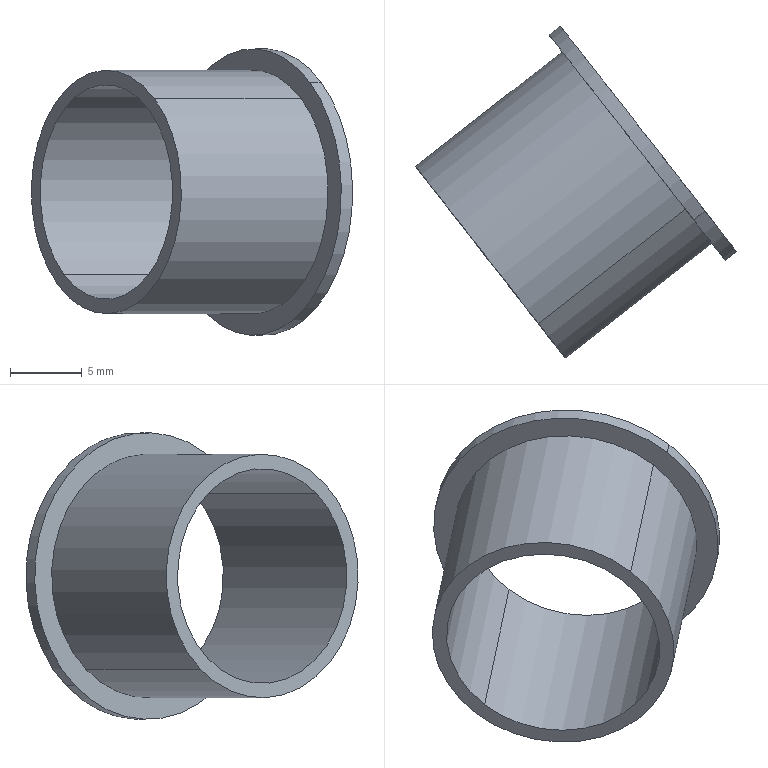Part | SolidWorks | features BaseBody 1 | 1 solid | 9 faces | box 22.422 x 23.197 x 20 mm | volume 790.896 mm3 | cylinder 6 | plane 3 | commonest cylinder face diameters 15 x2 17 x2 20 x2
STEP:
#1=CARTESIAN_POINT('',(6.767,90.458,77.91));
#2=VERTEX_POINT('',#1);
#3=CARTESIAN_POINT('',(-1.148,100.588,62.59));
#4=VERTEX_POINT('',#3);
#5=CARTESIAN_POINT('',(2.809,95.523,70.25));
#6=DIRECTION('',(-0.788,-0.6157,0.));
#7=DIRECTION('',(0.3957,-0.5065,0.766));
#8=AXIS2_PLACEMENT_3D('',#5,#6,#7);
#9=CIRCLE('',#8,10.);
#10=EDGE_CURVE('',#2,#4,#9,.T.);
#11=ORIENTED_EDGE('',*,*,#10,.F.);
#12=CARTESIAN_POINT('',(7.555,91.074,77.91));
#13=VERTEX_POINT('',#12);
#14=CARTESIAN_POINT('',(6.767,90.458,77.91));
#15=DIRECTION('',(0.788,0.6157,0.));
#16=VECTOR('',#15,1000.);
#17=LINE('',#14,#16);
#18=EDGE_CURVE('',#2,#13,#17,.T.);
#19=ORIENTED_EDGE('',*,*,#18,.T.);
#20=CARTESIAN_POINT('',(-0.36,101.204,62.59));
#21=VERTEX_POINT('',#20);
#22=CARTESIAN_POINT('',(3.597,96.139,70.25));
#23=DIRECTION('',(-0.788,-0.6157,0.));
#24=DIRECTION('',(0.3957,-0.5065,0.766));
#25=AXIS2_PLACEMENT_3D('',#22,#23,#24);
#26=CIRCLE('',#25,10.);
#27=EDGE_CURVE('',#13,#21,#26,.T.);
#28=ORIENTED_EDGE('',*,*,#27,.T.);
#29=CARTESIAN_POINT('',(-1.148,100.588,62.59));
#30=DIRECTION('',(0.788,0.6157,0.));
#31=VECTOR('',#30,1000.);
#32=LINE('',#29,#31);
#33=EDGE_CURVE('',#4,#21,#32,.T.);
#34=ORIENTED_EDGE('',*,*,#33,.F.);
#35=EDGE_LOOP('',(#11,#19,#28,#34));
#36=FACE_OUTER_BOUND('',#35,.T.);
#37=CARTESIAN_POINT('',(2.809,95.523,70.25));
#38=DIRECTION('',(0.788,0.6157,0.));
#39=DIRECTION('',(-0.3957,0.5065,-0.766));
#40=AXIS2_PLACEMENT_3D('',#37,#38,#39);
#41=CYLINDRICAL_SURFACE('',#40,10.);
#42=ADVANCED_FACE('',(#36),#41,.T.);
#43=CARTESIAN_POINT('',(-4.071,83.214,76.761));
#44=VERTEX_POINT('',#43);
#45=CARTESIAN_POINT('',(-10.799,91.825,63.739));
#46=VERTEX_POINT('',#45);
#47=CARTESIAN_POINT('',(-7.435,87.52,70.25));
#48=DIRECTION('',(-0.788,-0.6157,0.));
#49=DIRECTION('',(0.3957,-0.5065,0.766));
#50=AXIS2_PLACEMENT_3D('',#47,#48,#49);
#51=CIRCLE('',#50,8.5);
#52=EDGE_CURVE('',#44,#46,#51,.T.);
#53=ORIENTED_EDGE('',*,*,#52,.F.);
#54=CARTESIAN_POINT('',(6.173,91.218,76.761));
#55=VERTEX_POINT('',#54);
#56=CARTESIAN_POINT('',(-4.071,83.214,76.761));
#57=DIRECTION('',(0.788,0.6157,0.));
#58=VECTOR('',#57,1000.);
#59=LINE('',#56,#58);
#60=EDGE_CURVE('',#44,#55,#59,.T.);
#61=ORIENTED_EDGE('',*,*,#60,.T.);
#62=CARTESIAN_POINT('',(-0.5544,99.829,63.739));
#63=VERTEX_POINT('',#62);
#64=CARTESIAN_POINT('',(2.809,95.523,70.25));
#65=DIRECTION('',(-0.788,-0.6157,0.));
#66=DIRECTION('',(0.3957,-0.5065,0.766));
#67=AXIS2_PLACEMENT_3D('',#64,#65,#66);
#68=CIRCLE('',#67,8.5);
#69=EDGE_CURVE('',#55,#63,#68,.T.);
#70=ORIENTED_EDGE('',*,*,#69,.T.);
#71=CARTESIAN_POINT('',(-10.799,91.825,63.739));
#72=DIRECTION('',(0.788,0.6157,0.));
#73=VECTOR('',#72,1000.);
#74=LINE('',#71,#73);
#75=EDGE_CURVE('',#46,#63,#74,.T.);
#76=ORIENTED_EDGE('',*,*,#75,.F.);
#77=EDGE_LOOP('',(#53,#61,#70,#76));
#78=FACE_OUTER_BOUND('',#77,.T.);
#79=CARTESIAN_POINT('',(-7.435,87.52,70.25));
#80=DIRECTION('',(0.788,0.6157,0.));
#81=DIRECTION('',(-0.3957,0.5065,-0.766));
#82=AXIS2_PLACEMENT_3D('',#79,#80,#81);
#83=CYLINDRICAL_SURFACE('',#82,8.5);
#84=ADVANCED_FACE('',(#78),#83,.T.);
#85=CARTESIAN_POINT('',(0.6293,99.938,64.505));
#86=VERTEX_POINT('',#85);
#87=CARTESIAN_POINT('',(6.565,92.34,75.995));
#88=VERTEX_POINT('',#87);
#89=CARTESIAN_POINT('',(3.597,96.139,70.25));
#90=DIRECTION('',(-0.788,-0.6157,0.));
#91=DIRECTION('',(0.3957,-0.5065,0.766));
#92=AXIS2_PLACEMENT_3D('',#89,#90,#91);
#93=CIRCLE('',#92,7.5);
#94=EDGE_CURVE('',#86,#88,#93,.T.);
#95=ORIENTED_EDGE('',*,*,#94,.F.);
#96=CARTESIAN_POINT('',(-10.403,91.319,64.505));
#97=VERTEX_POINT('',#96);
#98=CARTESIAN_POINT('',(0.6293,99.938,64.505));
#99=DIRECTION('',(-0.788,-0.6157,0.));
#100=VECTOR('',#99,1000.);
#101=LINE('',#98,#100);
#102=EDGE_CURVE('',#86,#97,#101,.T.);
#103=ORIENTED_EDGE('',*,*,#102,.T.);
#104=CARTESIAN_POINT('',(-4.467,83.721,75.995));
#105=VERTEX_POINT('',#104);
#106=CARTESIAN_POINT('',(-7.435,87.52,70.25));
#107=DIRECTION('',(-0.788,-0.6157,0.));
#108=DIRECTION('',(0.3957,-0.5065,0.766));
#109=AXIS2_PLACEMENT_3D('',#106,#107,#108);
#110=CIRCLE('',#109,7.5);
#111=EDGE_CURVE('',#97,#105,#110,.T.);
#112=ORIENTED_EDGE('',*,*,#111,.T.);
#113=CARTESIAN_POINT('',(6.565,92.34,75.995));
#114=DIRECTION('',(-0.788,-0.6157,0.));
#115=VECTOR('',#114,1000.);
#116=LINE('',#113,#115);
#117=EDGE_CURVE('',#88,#105,#116,.T.);
#118=ORIENTED_EDGE('',*,*,#117,.F.);
#119=EDGE_LOOP('',(#95,#103,#112,#118));
#120=FACE_OUTER_BOUND('',#119,.T.);
#121=CARTESIAN_POINT('',(3.597,96.139,70.25));
#122=DIRECTION('',(-0.788,-0.6157,0.));
#123=DIRECTION('',(0.3957,-0.5065,0.766));
#124=AXIS2_PLACEMENT_3D('',#121,#122,#123);
#125=CYLINDRICAL_SURFACE('',#124,7.5);
#126=ADVANCED_FACE('',(#120),#125,.F.);
#127=ORIENTED_EDGE('',*,*,#102,.F.);
#128=CARTESIAN_POINT('',(3.597,96.139,70.25));
#129=DIRECTION('',(-0.788,-0.6157,0.));
#130=DIRECTION('',(0.3957,-0.5065,0.766));
#131=AXIS2_PLACEMENT_3D('',#128,#129,#130);
#132=CIRCLE('',#131,7.5);
#133=EDGE_CURVE('',#88,#86,#132,.T.);
#134=ORIENTED_EDGE('',*,*,#133,.F.);
#135=ORIENTED_EDGE('',*,*,#117,.T.);
#136=CARTESIAN_POINT('',(-7.435,87.52,70.25));
#137=DIRECTION('',(-0.788,-0.6157,0.));
#138=DIRECTION('',(0.3957,-0.5065,0.766));
#139=AXIS2_PLACEMENT_3D('',#136,#137,#138);
#140=CIRCLE('',#139,7.5);
#141=EDGE_CURVE('',#105,#97,#140,.T.);
#142=ORIENTED_EDGE('',*,*,#141,.T.);
#143=EDGE_LOOP('',(#127,#134,#135,#142));
#144=FACE_OUTER_BOUND('',#143,.T.);
#145=CARTESIAN_POINT('',(3.597,96.139,70.25));
#146=DIRECTION('',(-0.788,-0.6157,0.));
#147=DIRECTION('',(0.3957,-0.5065,0.766));
#148=AXIS2_PLACEMENT_3D('',#145,#146,#147);
#149=CYLINDRICAL_SURFACE('',#148,7.5);
#150=ADVANCED_FACE('',(#144),#149,.F.);
#151=CARTESIAN_POINT('',(-7.435,87.52,70.25));
#152=DIRECTION('',(-0.788,-0.6157,0.));
#153=DIRECTION('',(0.3957,-0.5065,0.766));
#154=AXIS2_PLACEMENT_3D('',#151,#152,#153);
#155=CIRCLE('',#154,8.5);
#156=EDGE_CURVE('',#46,#44,#155,.T.);
#157=ORIENTED_EDGE('',*,*,#156,.T.);
#158=ORIENTED_EDGE('',*,*,#52,.T.);
#159=EDGE_LOOP('',(#157,#158));
#160=FACE_OUTER_BOUND('',#159,.T.);
#161=ORIENTED_EDGE('',*,*,#141,.F.);
#162=ORIENTED_EDGE('',*,*,#111,.F.);
#163=EDGE_LOOP('',(#161,#162));
#164=FACE_BOUND('',#163,.T.);
#165=CARTESIAN_POINT('',(-7.435,87.52,70.25));
#166=DIRECTION('',(-0.788,-0.6157,0.));
#167=DIRECTION('',(-0.6157,0.788,0.));
#168=AXIS2_PLACEMENT_3D('',#165,#166,#167);
#169=PLANE('',#168);
#170=ADVANCED_FACE('',(#160,#164),#169,.T.);
#171=ORIENTED_EDGE('',*,*,#60,.F.);
#172=ORIENTED_EDGE('',*,*,#156,.F.);
#173=ORIENTED_EDGE('',*,*,#75,.T.);
#174=CARTESIAN_POINT('',(2.809,95.523,70.25));
#175=DIRECTION('',(-0.788,-0.6157,0.));
#176=DIRECTION('',(0.3957,-0.5065,0.766));
#177=AXIS2_PLACEMENT_3D('',#174,#175,#176);
#178=CIRCLE('',#177,8.5);
#179=EDGE_CURVE('',#63,#55,#178,.T.);
#180=ORIENTED_EDGE('',*,*,#179,.T.);
#181=EDGE_LOOP('',(#171,#172,#173,#180));
#182=FACE_OUTER_BOUND('',#181,.T.);
#183=CARTESIAN_POINT('',(-7.435,87.52,70.25));
#184=DIRECTION('',(0.788,0.6157,0.));
#185=DIRECTION('',(-0.3957,0.5065,-0.766));
#186=AXIS2_PLACEMENT_3D('',#183,#184,#185);
#187=CYLINDRICAL_SURFACE('',#186,8.5);
#188=ADVANCED_FACE('',(#182),#187,.T.);
#189=CARTESIAN_POINT('',(3.597,96.139,70.25));
#190=DIRECTION('',(-0.788,-0.6157,0.));
#191=DIRECTION('',(0.3957,-0.5065,0.766));
#192=AXIS2_PLACEMENT_3D('',#189,#190,#191);
#193=CIRCLE('',#192,10.);
#194=EDGE_CURVE('',#21,#13,#193,.T.);
#195=ORIENTED_EDGE('',*,*,#194,.F.);
#196=ORIENTED_EDGE('',*,*,#27,.F.);
#197=EDGE_LOOP('',(#195,#196));
#198=FACE_OUTER_BOUND('',#197,.T.);
#199=ORIENTED_EDGE('',*,*,#133,.T.);
#200=ORIENTED_EDGE('',*,*,#94,.T.);
#201=EDGE_LOOP('',(#199,#200));
#202=FACE_BOUND('',#201,.T.);
#203=CARTESIAN_POINT('',(3.597,96.139,70.25));
#204=DIRECTION('',(-0.788,-0.6157,0.));
#205=DIRECTION('',(-0.6157,0.788,0.));
#206=AXIS2_PLACEMENT_3D('',#203,#204,#205);
#207=PLANE('',#206);
#208=ADVANCED_FACE('',(#198,#202),#207,.F.);
#209=ORIENTED_EDGE('',*,*,#18,.F.);
#210=CARTESIAN_POINT('',(2.809,95.523,70.25));
#211=DIRECTION('',(-0.788,-0.6157,0.));
#212=DIRECTION('',(0.3957,-0.5065,0.766));
#213=AXIS2_PLACEMENT_3D('',#210,#211,#212);
#214=CIRCLE('',#213,10.);
#215=EDGE_CURVE('',#4,#2,#214,.T.);
#216=ORIENTED_EDGE('',*,*,#215,.F.);
#217=ORIENTED_EDGE('',*,*,#33,.T.);
#218=ORIENTED_EDGE('',*,*,#194,.T.);
#219=EDGE_LOOP('',(#209,#216,#217,#218));
#220=FACE_OUTER_BOUND('',#219,.T.);
#221=CARTESIAN_POINT('',(2.809,95.523,70.25));
#222=DIRECTION('',(0.788,0.6157,0.));
#223=DIRECTION('',(-0.3957,0.5065,-0.766));
#224=AXIS2_PLACEMENT_3D('',#221,#222,#223);
#225=CYLINDRICAL_SURFACE('',#224,10.);
#226=ADVANCED_FACE('',(#220),#225,.T.);
#227=ORIENTED_EDGE('',*,*,#179,.F.);
#228=ORIENTED_EDGE('',*,*,#69,.F.);
#229=EDGE_LOOP('',(#227,#228));
#230=FACE_BOUND('',#229,.T.);
#231=ORIENTED_EDGE('',*,*,#215,.T.);
#232=ORIENTED_EDGE('',*,*,#10,.T.);
#233=EDGE_LOOP('',(#231,#232));
#234=FACE_OUTER_BOUND('',#233,.T.);
#235=CARTESIAN_POINT('',(2.809,95.523,70.25));
#236=DIRECTION('',(-0.788,-0.6157,0.));
#237=DIRECTION('',(-0.6157,0.788,0.));
#238=AXIS2_PLACEMENT_3D('',#235,#236,#237);
#239=PLANE('',#238);
#240=ADVANCED_FACE('',(#230,#234),#239,.T.);
#241=CLOSED_SHELL('',(#42,#84,#126,#150,#170,#188,#208,#226,#240));
#242=MANIFOLD_SOLID_BREP('',#241);
#243=CARTESIAN_POINT('',(0.,0.,0.));
#244=DIRECTION('',(0.,0.,1.));
#245=DIRECTION('',(1.,0.,0.));
#246=AXIS2_PLACEMENT_3D('',#243,#244,#245);
#247=(LENGTH_UNIT()NAMED_UNIT(*)SI_UNIT(.MILLI.,.METRE.));
#248=UNCERTAINTY_MEASURE_WITH_UNIT(LENGTH_MEASURE(0.00001),#247,'','');
#249=(NAMED_UNIT(*)PLANE_ANGLE_UNIT()SI_UNIT($,.RADIAN.));
#250=(NAMED_UNIT(*)SI_UNIT($,.STERADIAN.)SOLID_ANGLE_UNIT());
#251=(GEOMETRIC_REPRESENTATION_CONTEXT(3)GLOBAL_UNCERTAINTY_ASSIGNED_CONTEXT((#248))GLOBAL_UNIT_ASSIGNED_CONTEXT((#247,#249,#250))REPRESENTATION_CONTEXT('',''));
#252=ADVANCED_BREP_SHAPE_REPRESENTATION('',(#242,#246),#251);